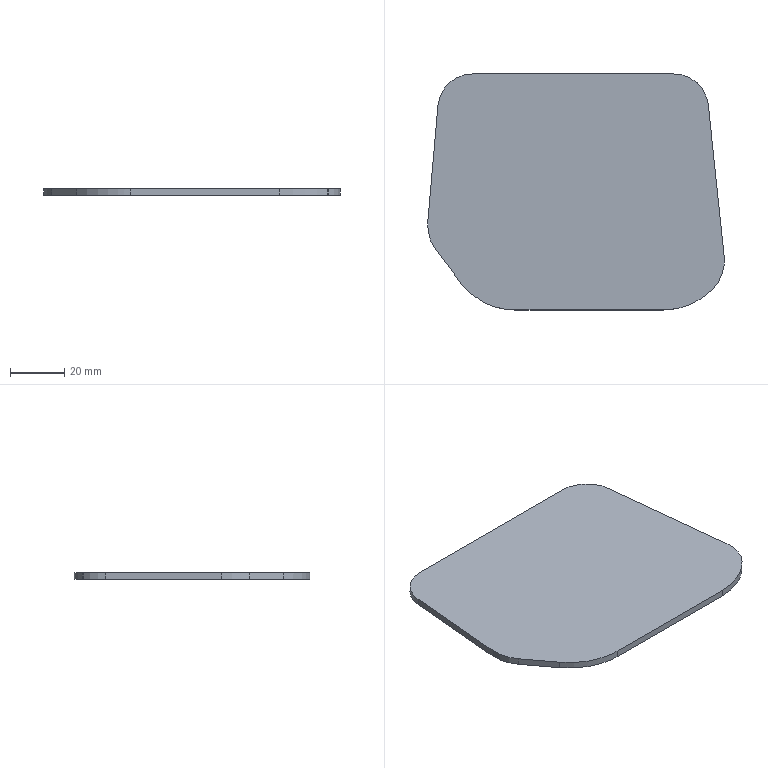Part | STEP file | lll_id402_x_t | 1 solid | 18 faces | box 109.864 x 87.36 x 2.5 mm | volume 21961 mm3 | plane 8 | cylinder 8 | other 2 | commonest cylinder face diameters 25.6 x4 30 x2 50 x2
STEP:
#1=CARTESIAN_POINT('',(3541.13,-66.264,0.00001757));
#2=VERTEX_POINT('',#1);
#3=CARTESIAN_POINT('',(3541.13,-66.264,-2.5));
#4=VERTEX_POINT('',#3);
#5=CARTESIAN_POINT('',(3541.13,-66.264,0.00001757));
#6=CARTESIAN_POINT('',(3541.13,-66.264,-0.8333));
#7=CARTESIAN_POINT('',(3541.13,-66.264,-1.667));
#8=CARTESIAN_POINT('',(3541.13,-66.264,-2.5));
#9=B_SPLINE_CURVE_WITH_KNOTS('',3,(#5,#6,#7,#8),.UNSPECIFIED.,.F.,.F.,(4,4),(0.,1.),.UNSPECIFIED.);
#10=EDGE_CURVE('',#2,#4,#9,.T.);
#11=ORIENTED_EDGE('',*,*,#10,.F.);
#12=CARTESIAN_POINT('',(3541.656,-65.782,0.00001757));
#13=VERTEX_POINT('',#12);
#14=CARTESIAN_POINT('',(3537.286,-74.341,0.00001754));
#15=CARTESIAN_POINT('',(3537.32,-73.947,0.00001754));
#16=CARTESIAN_POINT('',(3537.425,-73.162,0.00001754));
#17=CARTESIAN_POINT('',(3537.778,-71.617,0.00001754));
#18=CARTESIAN_POINT('',(3538.492,-69.763,0.00001755));
#19=CARTESIAN_POINT('',(3539.736,-67.729,0.00001755));
#20=CARTESIAN_POINT('',(3541.341,-65.967,0.00001757));
#21=CARTESIAN_POINT('',(3543.237,-64.521,0.00001758));
#22=CARTESIAN_POINT('',(3545.372,-63.46,0.0000176));
#23=CARTESIAN_POINT('',(3547.281,-62.91,0.00001761));
#24=CARTESIAN_POINT('',(3548.85,-62.692,0.00001762));
#25=CARTESIAN_POINT('',(3549.641,-62.657,0.00001763));
#26=CARTESIAN_POINT('',(3550.037,-62.657,0.00001763));
#27=B_SPLINE_CURVE_WITH_KNOTS('',3,(#14,#15,#16,#17,#18,#19,#20,#21,#22,#23,#24,#25,#26),.UNSPECIFIED.,.F.,.F.,(4,1,1,1,1,1,1,1,1,1,4),(0.,0.0625,0.125,0.25,0.375,0.5,0.625,0.75,0.875,0.9375,1.),.UNSPECIFIED.);
#28=EDGE_CURVE('',#2,#13,#27,.T.);
#29=ORIENTED_EDGE('',*,*,#28,.T.);
#30=CARTESIAN_POINT('',(3541.656,-65.782,-2.5));
#31=VERTEX_POINT('',#30);
#32=CARTESIAN_POINT('',(3541.656,-65.782,-2.5));
#33=CARTESIAN_POINT('',(3541.656,-65.782,-1.667));
#34=CARTESIAN_POINT('',(3541.656,-65.782,-0.8333));
#35=CARTESIAN_POINT('',(3541.656,-65.782,0.00001757));
#36=B_SPLINE_CURVE_WITH_KNOTS('',3,(#32,#33,#34,#35),.UNSPECIFIED.,.F.,.F.,(4,4),(0.,1.),.UNSPECIFIED.);
#37=EDGE_CURVE('',#31,#13,#36,.T.);
#38=ORIENTED_EDGE('',*,*,#37,.F.);
#39=CARTESIAN_POINT('',(3537.286,-74.341,-2.5));
#40=CARTESIAN_POINT('',(3537.32,-73.947,-2.5));
#41=CARTESIAN_POINT('',(3537.425,-73.162,-2.5));
#42=CARTESIAN_POINT('',(3537.778,-71.617,-2.5));
#43=CARTESIAN_POINT('',(3538.492,-69.763,-2.5));
#44=CARTESIAN_POINT('',(3539.736,-67.729,-2.5));
#45=CARTESIAN_POINT('',(3541.341,-65.967,-2.5));
#46=CARTESIAN_POINT('',(3543.237,-64.521,-2.5));
#47=CARTESIAN_POINT('',(3545.372,-63.46,-2.5));
#48=CARTESIAN_POINT('',(3547.281,-62.91,-2.5));
#49=CARTESIAN_POINT('',(3548.85,-62.692,-2.5));
#50=CARTESIAN_POINT('',(3549.641,-62.657,-2.5));
#51=CARTESIAN_POINT('',(3550.037,-62.657,-2.5));
#52=B_SPLINE_CURVE_WITH_KNOTS('',3,(#39,#40,#41,#42,#43,#44,#45,#46,#47,#48,#49,#50,#51),.UNSPECIFIED.,.F.,.F.,(4,1,1,1,1,1,1,1,1,1,4),(0.,0.0625,0.125,0.25,0.375,0.5,0.625,0.75,0.875,0.9375,1.),.UNSPECIFIED.);
#53=EDGE_CURVE('',#4,#31,#52,.T.);
#54=ORIENTED_EDGE('',*,*,#53,.F.);
#55=EDGE_LOOP('',(#11,#29,#38,#54));
#56=FACE_OUTER_BOUND('',#55,.T.);
#57=CARTESIAN_POINT('',(3537.286,-74.341,-2.5));
#58=CARTESIAN_POINT('',(3537.32,-73.947,-2.5));
#59=CARTESIAN_POINT('',(3537.425,-73.162,-2.5));
#60=CARTESIAN_POINT('',(3537.778,-71.617,-2.5));
#61=CARTESIAN_POINT('',(3538.492,-69.763,-2.5));
#62=CARTESIAN_POINT('',(3539.736,-67.729,-2.5));
#63=CARTESIAN_POINT('',(3541.341,-65.967,-2.5));
#64=CARTESIAN_POINT('',(3543.237,-64.521,-2.5));
#65=CARTESIAN_POINT('',(3545.372,-63.46,-2.5));
#66=CARTESIAN_POINT('',(3547.281,-62.91,-2.5));
#67=CARTESIAN_POINT('',(3548.85,-62.692,-2.5));
#68=CARTESIAN_POINT('',(3549.641,-62.657,-2.5));
#69=CARTESIAN_POINT('',(3550.037,-62.657,-2.5));
#70=B_SPLINE_CURVE_WITH_KNOTS('',3,(#57,#58,#59,#60,#61,#62,#63,#64,#65,#66,#67,#68,#69),.UNSPECIFIED.,.F.,.F.,(4,1,1,1,1,1,1,1,1,1,4),(0.,0.0625,0.125,0.25,0.375,0.5,0.625,0.75,0.875,0.9375,1.),.UNSPECIFIED.);
#71=DIRECTION('',(0.,0.000000006,1.));
#72=VECTOR('',#71,1.);
#73=SURFACE_OF_LINEAR_EXTRUSION('',#70,#72);
#74=ADVANCED_FACE('',(#56),#73,.F.);
#75=CARTESIAN_POINT('',(3632.944,-65.718,0.00001826));
#76=VERTEX_POINT('',#75);
#77=CARTESIAN_POINT('',(3632.944,-65.718,-2.5));
#78=VERTEX_POINT('',#77);
#79=CARTESIAN_POINT('',(3632.944,-65.718,0.00001826));
#80=CARTESIAN_POINT('',(3632.944,-65.718,-0.8333));
#81=CARTESIAN_POINT('',(3632.944,-65.718,-1.667));
#82=CARTESIAN_POINT('',(3632.944,-65.718,-2.5));
#83=B_SPLINE_CURVE_WITH_KNOTS('',3,(#79,#80,#81,#82),.UNSPECIFIED.,.F.,.F.,(4,4),(0.,1.),.UNSPECIFIED.);
#84=EDGE_CURVE('',#76,#78,#83,.T.);
#85=ORIENTED_EDGE('',*,*,#84,.F.);
#86=CARTESIAN_POINT('',(3633.454,-66.177,0.00001826));
#87=VERTEX_POINT('',#86);
#88=CARTESIAN_POINT('',(3624.637,-62.657,0.0000182));
#89=CARTESIAN_POINT('',(3625.028,-62.657,0.0000182));
#90=CARTESIAN_POINT('',(3625.81,-62.691,0.00001821));
#91=CARTESIAN_POINT('',(3627.361,-62.904,0.00001822));
#92=CARTESIAN_POINT('',(3629.249,-63.441,0.00001823));
#93=CARTESIAN_POINT('',(3631.364,-64.478,0.00001825));
#94=CARTESIAN_POINT('',(3633.249,-65.892,0.00001826));
#95=CARTESIAN_POINT('',(3634.852,-67.618,0.00001828));
#96=CARTESIAN_POINT('',(3636.105,-69.613,0.00001828));
#97=CARTESIAN_POINT('',(3636.836,-71.435,0.00001829));
#98=CARTESIAN_POINT('',(3637.21,-72.956,0.00001829));
#99=CARTESIAN_POINT('',(3637.326,-73.73,0.00001829));
#100=CARTESIAN_POINT('',(3637.367,-74.119,0.00001829));
#101=B_SPLINE_CURVE_WITH_KNOTS('',3,(#88,#89,#90,#91,#92,#93,#94,#95,#96,#97,#98,#99,#100),.UNSPECIFIED.,.F.,.F.,(4,1,1,1,1,1,1,1,1,1,4),(0.,0.0625,0.125,0.25,0.375,0.5,0.625,0.75,0.875,0.9375,1.),.UNSPECIFIED.);
#102=EDGE_CURVE('',#76,#87,#101,.T.);
#103=ORIENTED_EDGE('',*,*,#102,.T.);
#104=CARTESIAN_POINT('',(3633.454,-66.177,-2.5));
#105=VERTEX_POINT('',#104);
#106=CARTESIAN_POINT('',(3633.454,-66.177,-2.5));
#107=CARTESIAN_POINT('',(3633.454,-66.177,-1.667));
#108=CARTESIAN_POINT('',(3633.454,-66.177,-0.8333));
#109=CARTESIAN_POINT('',(3633.454,-66.177,0.00001826));
#110=B_SPLINE_CURVE_WITH_KNOTS('',3,(#106,#107,#108,#109),.UNSPECIFIED.,.F.,.F.,(4,4),(0.,1.),.UNSPECIFIED.);
#111=EDGE_CURVE('',#105,#87,#110,.T.);
#112=ORIENTED_EDGE('',*,*,#111,.F.);
#113=CARTESIAN_POINT('',(3624.637,-62.657,-2.5));
#114=CARTESIAN_POINT('',(3625.028,-62.657,-2.5));
#115=CARTESIAN_POINT('',(3625.81,-62.691,-2.5));
#116=CARTESIAN_POINT('',(3627.361,-62.904,-2.5));
#117=CARTESIAN_POINT('',(3629.249,-63.441,-2.5));
#118=CARTESIAN_POINT('',(3631.364,-64.478,-2.5));
#119=CARTESIAN_POINT('',(3633.249,-65.892,-2.5));
#120=CARTESIAN_POINT('',(3634.852,-67.618,-2.5));
#121=CARTESIAN_POINT('',(3636.105,-69.613,-2.5));
#122=CARTESIAN_POINT('',(3636.836,-71.435,-2.5));
#123=CARTESIAN_POINT('',(3637.21,-72.956,-2.5));
#124=CARTESIAN_POINT('',(3637.326,-73.73,-2.5));
#125=CARTESIAN_POINT('',(3637.367,-74.119,-2.5));
#126=B_SPLINE_CURVE_WITH_KNOTS('',3,(#113,#114,#115,#116,#117,#118,#119,#120,#121,#122,#123,#124,#125),.UNSPECIFIED.,.F.,.F.,(4,1,1,1,1,1,1,1,1,1,4),(0.,0.0625,0.125,0.25,0.375,0.5,0.625,0.75,0.875,0.9375,1.),.UNSPECIFIED.);
#127=EDGE_CURVE('',#78,#105,#126,.T.);
#128=ORIENTED_EDGE('',*,*,#127,.F.);
#129=EDGE_LOOP('',(#85,#103,#112,#128));
#130=FACE_OUTER_BOUND('',#129,.T.);
#131=CARTESIAN_POINT('',(3624.637,-62.657,-2.5));
#132=CARTESIAN_POINT('',(3625.028,-62.657,-2.5));
#133=CARTESIAN_POINT('',(3625.81,-62.691,-2.5));
#134=CARTESIAN_POINT('',(3627.361,-62.904,-2.5));
#135=CARTESIAN_POINT('',(3629.249,-63.441,-2.5));
#136=CARTESIAN_POINT('',(3631.364,-64.478,-2.5));
#137=CARTESIAN_POINT('',(3633.249,-65.892,-2.5));
#138=CARTESIAN_POINT('',(3634.852,-67.618,-2.5));
#139=CARTESIAN_POINT('',(3636.105,-69.613,-2.5));
#140=CARTESIAN_POINT('',(3636.836,-71.435,-2.5));
#141=CARTESIAN_POINT('',(3637.21,-72.956,-2.5));
#142=CARTESIAN_POINT('',(3637.326,-73.73,-2.5));
#143=CARTESIAN_POINT('',(3637.367,-74.119,-2.5));
#144=B_SPLINE_CURVE_WITH_KNOTS('',3,(#131,#132,#133,#134,#135,#136,#137,#138,#139,#140,#141,#142,#143),.UNSPECIFIED.,.F.,.F.,(4,1,1,1,1,1,1,1,1,1,4),(0.,0.0625,0.125,0.25,0.375,0.5,0.625,0.75,0.875,0.9375,1.),.UNSPECIFIED.);
#145=DIRECTION('',(0.,0.000000006,1.));
#146=VECTOR('',#145,1.);
#147=SURFACE_OF_LINEAR_EXTRUSION('',#144,#146);
#148=ADVANCED_FACE('',(#130),#147,.F.);
#149=CARTESIAN_POINT('',(3643.25,-130.089,-2.5));
#150=VERTEX_POINT('',#149);
#151=CARTESIAN_POINT('',(3643.25,-130.089,0.00001832));
#152=VERTEX_POINT('',#151);
#153=CARTESIAN_POINT('',(3643.25,-130.089,-7.5));
#154=DIRECTION('',(0.000000001,0.000000001,1.));
#155=VECTOR('',#154,1.);
#156=LINE('',#153,#155);
#157=EDGE_CURVE('',#150,#152,#156,.T.);
#158=ORIENTED_EDGE('',*,*,#157,.F.);
#159=CARTESIAN_POINT('',(3637.367,-74.119,-2.5));
#160=VERTEX_POINT('',#159);
#161=CARTESIAN_POINT('',(3639.152,-91.104,-2.5));
#162=DIRECTION('',(0.1045,-0.9945,0.000000001));
#163=VECTOR('',#162,1.);
#164=LINE('',#161,#163);
#165=EDGE_CURVE('',#160,#150,#164,.T.);
#166=ORIENTED_EDGE('',*,*,#165,.F.);
#167=CARTESIAN_POINT('',(3637.367,-74.119,0.0000182));
#168=VERTEX_POINT('',#167);
#169=CARTESIAN_POINT('',(3637.367,-74.119,-2.5));
#170=DIRECTION('',(0.,0.000000006,1.));
#171=VECTOR('',#170,1.);
#172=LINE('',#169,#171);
#173=EDGE_CURVE('',#160,#168,#172,.T.);
#174=ORIENTED_EDGE('',*,*,#173,.T.);
#175=CARTESIAN_POINT('',(3639.152,-91.104,0.00001831));
#176=DIRECTION('',(0.1045,-0.9945,0.000000001));
#177=VECTOR('',#176,1.);
#178=LINE('',#175,#177);
#179=EDGE_CURVE('',#168,#152,#178,.T.);
#180=ORIENTED_EDGE('',*,*,#179,.T.);
#181=EDGE_LOOP('',(#158,#166,#174,#180));
#182=FACE_OUTER_BOUND('',#181,.T.);
#183=CARTESIAN_POINT('',(3637.367,-74.119,-2.5));
#184=DIRECTION('',(-0.9945,-0.1045,0.000000001));
#185=DIRECTION('',(0.1045,-0.9945,0.));
#186=AXIS2_PLACEMENT_3D('',#183,#184,#185);
#187=PLANE('',#186);
#188=ADVANCED_FACE('',(#182),#187,.F.);
#189=CARTESIAN_POINT('',(3637.367,-74.119,-2.5));
#190=CARTESIAN_POINT('',(3637.052,-71.122,-2.5));
#191=CARTESIAN_POINT('',(3635.638,-68.253,-2.5));
#192=CARTESIAN_POINT('',(3633.454,-66.177,-2.5));
#193=B_SPLINE_CURVE_WITH_KNOTS('',3,(#189,#190,#191,#192),.UNSPECIFIED.,.F.,.F.,(4,4),(0.,1.),.UNSPECIFIED.);
#194=EDGE_CURVE('',#160,#105,#193,.T.);
#195=ORIENTED_EDGE('',*,*,#194,.F.);
#196=ORIENTED_EDGE('',*,*,#165,.T.);
#197=CARTESIAN_POINT('',(3638.938,-142.263,-2.5));
#198=VERTEX_POINT('',#197);
#199=CARTESIAN_POINT('',(3628.332,-131.657,-2.5));
#200=DIRECTION('',(-0.000000008,0.,1.));
#201=DIRECTION('',(1.,0.,0.000000008));
#202=AXIS2_PLACEMENT_3D('',#199,#200,#201);
#203=CIRCLE('',#202,15.);
#204=EDGE_CURVE('',#198,#150,#203,.T.);
#205=ORIENTED_EDGE('',*,*,#204,.F.);
#206=CARTESIAN_POINT('',(3638.507,-142.694,-2.5));
#207=VERTEX_POINT('',#206);
#208=CARTESIAN_POINT('',(3596.229,-184.973,-2.5));
#209=DIRECTION('',(0.7071,0.7071,0.000000005));
#210=VECTOR('',#209,1.);
#211=LINE('',#208,#210);
#212=EDGE_CURVE('',#207,#198,#211,.T.);
#213=ORIENTED_EDGE('',*,*,#212,.F.);
#214=CARTESIAN_POINT('',(3620.83,-150.017,-2.5));
#215=VERTEX_POINT('',#214);
#216=CARTESIAN_POINT('',(3620.83,-125.017,-2.5));
#217=DIRECTION('',(-0.000000008,0.,1.));
#218=DIRECTION('',(1.,0.,0.000000008));
#219=AXIS2_PLACEMENT_3D('',#216,#217,#218);
#220=CIRCLE('',#219,25.);
#221=EDGE_CURVE('',#215,#207,#220,.T.);
#222=ORIENTED_EDGE('',*,*,#221,.F.);
#223=CARTESIAN_POINT('',(3565.78,-150.017,-2.5));
#224=VERTEX_POINT('',#223);
#225=CARTESIAN_POINT('',(3581.149,-150.017,-2.5));
#226=DIRECTION('',(-1.,0.,-0.000000008));
#227=VECTOR('',#226,1.);
#228=LINE('',#225,#227);
#229=EDGE_CURVE('',#215,#224,#228,.T.);
#230=ORIENTED_EDGE('',*,*,#229,.T.);
#231=CARTESIAN_POINT('',(3545.814,-140.062,-2.5));
#232=VERTEX_POINT('',#231);
#233=CARTESIAN_POINT('',(3545.814,-140.062,-2.5));
#234=CARTESIAN_POINT('',(3548.134,-143.14,-2.5));
#235=CARTESIAN_POINT('',(3551.176,-145.67,-2.5));
#236=CARTESIAN_POINT('',(3558.074,-149.11,-2.5));
#237=CARTESIAN_POINT('',(3561.926,-150.017,-2.5));
#238=CARTESIAN_POINT('',(3565.78,-150.017,-2.5));
#239=B_SPLINE_CURVE_WITH_KNOTS('',3,(#233,#234,#235,#236,#237,#238),.UNSPECIFIED.,.F.,.F.,(4,2,4),(0.,0.5,1.),.UNSPECIFIED.);
#240=EDGE_CURVE('',#232,#224,#239,.T.);
#241=ORIENTED_EDGE('',*,*,#240,.F.);
#242=CARTESIAN_POINT('',(3536.486,-127.684,-2.5));
#243=VERTEX_POINT('',#242);
#244=CARTESIAN_POINT('',(3541.15,-133.873,-2.5));
#245=DIRECTION('',(-0.6018,0.7986,-0.000000005));
#246=VECTOR('',#245,1.);
#247=LINE('',#244,#246);
#248=EDGE_CURVE('',#232,#243,#247,.T.);
#249=ORIENTED_EDGE('',*,*,#248,.T.);
#250=CARTESIAN_POINT('',(3533.523,-117.349,-2.5));
#251=VERTEX_POINT('',#250);
#252=CARTESIAN_POINT('',(3533.523,-117.349,-2.5));
#253=CARTESIAN_POINT('',(3533.204,-121.,-2.5));
#254=CARTESIAN_POINT('',(3534.281,-124.757,-2.5));
#255=CARTESIAN_POINT('',(3536.486,-127.684,-2.5));
#256=B_SPLINE_CURVE_WITH_KNOTS('',3,(#252,#253,#254,#255),.UNSPECIFIED.,.F.,.F.,(4,4),(0.,1.),.UNSPECIFIED.);
#257=EDGE_CURVE('',#251,#243,#256,.T.);
#258=ORIENTED_EDGE('',*,*,#257,.F.);
#259=CARTESIAN_POINT('',(3537.286,-74.341,-2.5));
#260=VERTEX_POINT('',#259);
#261=CARTESIAN_POINT('',(3535.404,-95.845,-2.5));
#262=DIRECTION('',(0.08716,0.9962,0.000000001));
#263=VECTOR('',#262,1.);
#264=LINE('',#261,#263);
#265=EDGE_CURVE('',#251,#260,#264,.T.);
#266=ORIENTED_EDGE('',*,*,#265,.T.);
#267=CARTESIAN_POINT('',(3541.13,-66.264,-2.5));
#268=CARTESIAN_POINT('',(3538.942,-68.384,-2.5));
#269=CARTESIAN_POINT('',(3537.551,-71.307,-2.5));
#270=CARTESIAN_POINT('',(3537.286,-74.341,-2.5));
#271=B_SPLINE_CURVE_WITH_KNOTS('',3,(#267,#268,#269,#270),.UNSPECIFIED.,.F.,.F.,(4,4),(0.,1.),.UNSPECIFIED.);
#272=EDGE_CURVE('',#4,#260,#271,.T.);
#273=ORIENTED_EDGE('',*,*,#272,.F.);
#274=ORIENTED_EDGE('',*,*,#53,.T.);
#275=CARTESIAN_POINT('',(3550.037,-62.657,-2.5));
#276=VERTEX_POINT('',#275);
#277=CARTESIAN_POINT('',(3550.037,-62.657,-2.5));
#278=CARTESIAN_POINT('',(3546.991,-62.657,-2.5));
#279=CARTESIAN_POINT('',(3543.958,-63.788,-2.5));
#280=CARTESIAN_POINT('',(3541.656,-65.782,-2.5));
#281=B_SPLINE_CURVE_WITH_KNOTS('',3,(#277,#278,#279,#280),.UNSPECIFIED.,.F.,.F.,(4,4),(0.,1.),.UNSPECIFIED.);
#282=EDGE_CURVE('',#276,#31,#281,.T.);
#283=ORIENTED_EDGE('',*,*,#282,.F.);
#284=CARTESIAN_POINT('',(3624.637,-62.657,-2.5));
#285=VERTEX_POINT('',#284);
#286=CARTESIAN_POINT('',(3587.337,-62.657,-2.5));
#287=DIRECTION('',(1.,0.,0.000000008));
#288=VECTOR('',#287,1.);
#289=LINE('',#286,#288);
#290=EDGE_CURVE('',#276,#285,#289,.T.);
#291=ORIENTED_EDGE('',*,*,#290,.T.);
#292=CARTESIAN_POINT('',(3632.944,-65.718,-2.5));
#293=CARTESIAN_POINT('',(3630.651,-63.763,-2.5));
#294=CARTESIAN_POINT('',(3627.65,-62.657,-2.5));
#295=CARTESIAN_POINT('',(3624.637,-62.657,-2.5));
#296=B_SPLINE_CURVE_WITH_KNOTS('',3,(#292,#293,#294,#295),.UNSPECIFIED.,.F.,.F.,(4,4),(0.,1.),.UNSPECIFIED.);
#297=EDGE_CURVE('',#78,#285,#296,.T.);
#298=ORIENTED_EDGE('',*,*,#297,.F.);
#299=ORIENTED_EDGE('',*,*,#127,.T.);
#300=EDGE_LOOP('',(#195,#196,#205,#213,#222,#230,#241,#249,#258,#266,#273,#274,#283,#291,#298,#299));
#301=FACE_OUTER_BOUND('',#300,.T.);
#302=CARTESIAN_POINT('',(3534.047,-122.791,-2.5));
#303=DIRECTION('',(-0.000000008,0.,1.));
#304=DIRECTION('',(-1.,0.,-0.000000008));
#305=AXIS2_PLACEMENT_3D('',#302,#303,#304);
#306=PLANE('',#305);
#307=ADVANCED_FACE('',(#301),#306,.F.);
#308=ORIENTED_EDGE('',*,*,#179,.F.);
#309=CARTESIAN_POINT('',(3637.367,-74.119,0.0000183));
#310=CARTESIAN_POINT('',(3637.051,-71.113,0.00001829));
#311=CARTESIAN_POINT('',(3635.645,-68.26,0.00001828));
#312=CARTESIAN_POINT('',(3633.454,-66.177,0.00001827));
#313=B_SPLINE_CURVE_WITH_KNOTS('',3,(#309,#310,#311,#312),.UNSPECIFIED.,.F.,.F.,(4,4),(0.,1.),.UNSPECIFIED.);
#314=EDGE_CURVE('',#168,#87,#313,.T.);
#315=ORIENTED_EDGE('',*,*,#314,.T.);
#316=ORIENTED_EDGE('',*,*,#102,.F.);
#317=CARTESIAN_POINT('',(3624.637,-62.657,0.0000182));
#318=VERTEX_POINT('',#317);
#319=CARTESIAN_POINT('',(3632.944,-65.718,0.00001826));
#320=CARTESIAN_POINT('',(3630.645,-63.757,0.00001824));
#321=CARTESIAN_POINT('',(3627.66,-62.657,0.00001822));
#322=CARTESIAN_POINT('',(3624.637,-62.657,0.0000182));
#323=B_SPLINE_CURVE_WITH_KNOTS('',3,(#319,#320,#321,#322),.UNSPECIFIED.,.F.,.F.,(4,4),(0.,1.),.UNSPECIFIED.);
#324=EDGE_CURVE('',#76,#318,#323,.T.);
#325=ORIENTED_EDGE('',*,*,#324,.T.);
#326=CARTESIAN_POINT('',(3550.037,-62.657,0.00001763));
#327=VERTEX_POINT('',#326);
#328=CARTESIAN_POINT('',(3587.337,-62.657,0.00001792));
#329=DIRECTION('',(1.,0.,0.000000008));
#330=VECTOR('',#329,1.);
#331=LINE('',#328,#330);
#332=EDGE_CURVE('',#327,#318,#331,.T.);
#333=ORIENTED_EDGE('',*,*,#332,.F.);
#334=CARTESIAN_POINT('',(3550.037,-62.657,0.00001763));
#335=CARTESIAN_POINT('',(3546.982,-62.657,0.00001761));
#336=CARTESIAN_POINT('',(3543.966,-63.781,0.00001759));
#337=CARTESIAN_POINT('',(3541.656,-65.782,0.00001757));
#338=B_SPLINE_CURVE_WITH_KNOTS('',3,(#334,#335,#336,#337),.UNSPECIFIED.,.F.,.F.,(4,4),(0.,1.),.UNSPECIFIED.);
#339=EDGE_CURVE('',#327,#13,#338,.T.);
#340=ORIENTED_EDGE('',*,*,#339,.T.);
#341=ORIENTED_EDGE('',*,*,#28,.F.);
#342=CARTESIAN_POINT('',(3537.286,-74.341,0.00001754));
#343=VERTEX_POINT('',#342);
#344=CARTESIAN_POINT('',(3541.13,-66.264,0.00001757));
#345=CARTESIAN_POINT('',(3538.936,-68.39,0.00001755));
#346=CARTESIAN_POINT('',(3537.552,-71.296,0.00001754));
#347=CARTESIAN_POINT('',(3537.286,-74.341,0.00001754));
#348=B_SPLINE_CURVE_WITH_KNOTS('',3,(#344,#345,#346,#347),.UNSPECIFIED.,.F.,.F.,(4,4),(0.,1.),.UNSPECIFIED.);
#349=EDGE_CURVE('',#2,#343,#348,.T.);
#350=ORIENTED_EDGE('',*,*,#349,.T.);
#351=CARTESIAN_POINT('',(3533.523,-117.349,0.00001762));
#352=VERTEX_POINT('',#351);
#353=CARTESIAN_POINT('',(3535.404,-95.845,0.00001752));
#354=DIRECTION('',(0.08716,0.9962,0.000000001));
#355=VECTOR('',#354,1.);
#356=LINE('',#353,#355);
#357=EDGE_CURVE('',#352,#343,#356,.T.);
#358=ORIENTED_EDGE('',*,*,#357,.F.);
#359=CARTESIAN_POINT('',(3536.486,-127.684,0.00001753));
#360=VERTEX_POINT('',#359);
#361=CARTESIAN_POINT('',(3533.523,-117.349,0.00001751));
#362=CARTESIAN_POINT('',(3533.203,-121.011,0.0000175));
#363=CARTESIAN_POINT('',(3534.273,-124.746,0.00001751));
#364=CARTESIAN_POINT('',(3536.486,-127.684,0.00001753));
#365=B_SPLINE_CURVE_WITH_KNOTS('',3,(#361,#362,#363,#364),.UNSPECIFIED.,.F.,.F.,(4,4),(0.,1.),.UNSPECIFIED.);
#366=EDGE_CURVE('',#352,#360,#365,.T.);
#367=ORIENTED_EDGE('',*,*,#366,.T.);
#368=CARTESIAN_POINT('',(3545.814,-140.062,0.00001775));
#369=VERTEX_POINT('',#368);
#370=CARTESIAN_POINT('',(3541.15,-133.873,0.00001757));
#371=DIRECTION('',(-0.6018,0.7986,-0.000000005));
#372=VECTOR('',#371,1.);
#373=LINE('',#370,#372);
#374=EDGE_CURVE('',#369,#360,#373,.T.);
#375=ORIENTED_EDGE('',*,*,#374,.F.);
#376=CARTESIAN_POINT('',(3565.78,-150.017,0.00001775));
#377=VERTEX_POINT('',#376);
#378=CARTESIAN_POINT('',(3545.814,-140.062,0.0000176));
#379=CARTESIAN_POINT('',(3548.144,-143.154,0.00001762));
#380=CARTESIAN_POINT('',(3551.161,-145.663,0.00001764));
#381=CARTESIAN_POINT('',(3558.089,-149.117,0.00001769));
#382=CARTESIAN_POINT('',(3561.907,-150.016,0.00001772));
#383=CARTESIAN_POINT('',(3565.78,-150.017,0.00001775));
#384=B_SPLINE_CURVE_WITH_KNOTS('',3,(#378,#379,#380,#381,#382,#383),.UNSPECIFIED.,.F.,.F.,(4,2,4),(0.,0.5,1.),.UNSPECIFIED.);
#385=EDGE_CURVE('',#369,#377,#384,.T.);
#386=ORIENTED_EDGE('',*,*,#385,.T.);
#387=CARTESIAN_POINT('',(3620.83,-150.017,0.00001817));
#388=VERTEX_POINT('',#387);
#389=CARTESIAN_POINT('',(3581.149,-150.017,0.00001787));
#390=DIRECTION('',(-1.,0.,-0.000000008));
#391=VECTOR('',#390,1.);
#392=LINE('',#389,#391);
#393=EDGE_CURVE('',#388,#377,#392,.T.);
#394=ORIENTED_EDGE('',*,*,#393,.F.);
#395=CARTESIAN_POINT('',(3638.507,-142.694,0.00001831));
#396=VERTEX_POINT('',#395);
#397=CARTESIAN_POINT('',(3620.83,-125.017,0.00001817));
#398=DIRECTION('',(0.000000008,0.,-1.));
#399=DIRECTION('',(1.,0.,0.000000008));
#400=AXIS2_PLACEMENT_3D('',#397,#398,#399);
#401=CIRCLE('',#400,25.);
#402=EDGE_CURVE('',#396,#388,#401,.T.);
#403=ORIENTED_EDGE('',*,*,#402,.F.);
#404=CARTESIAN_POINT('',(3638.938,-142.263,0.00001831));
#405=VERTEX_POINT('',#404);
#406=CARTESIAN_POINT('',(3596.229,-184.973,0.00001798));
#407=DIRECTION('',(0.7071,0.7071,0.000000005));
#408=VECTOR('',#407,1.);
#409=LINE('',#406,#408);
#410=EDGE_CURVE('',#396,#405,#409,.T.);
#411=ORIENTED_EDGE('',*,*,#410,.T.);
#412=CARTESIAN_POINT('',(3628.332,-131.657,0.00001823));
#413=DIRECTION('',(-0.000000008,0.,1.));
#414=DIRECTION('',(1.,0.,0.000000008));
#415=AXIS2_PLACEMENT_3D('',#412,#413,#414);
#416=CIRCLE('',#415,15.);
#417=EDGE_CURVE('',#405,#152,#416,.T.);
#418=ORIENTED_EDGE('',*,*,#417,.T.);
#419=EDGE_LOOP('',(#308,#315,#316,#325,#333,#340,#341,#350,#358,#367,#375,#386,#394,#403,#411,#418));
#420=FACE_OUTER_BOUND('',#419,.T.);
#421=CARTESIAN_POINT('',(3534.047,-122.791,0.00001751));
#422=DIRECTION('',(-0.000000008,0.,1.));
#423=DIRECTION('',(-1.,0.,-0.000000008));
#424=AXIS2_PLACEMENT_3D('',#421,#422,#423);
#425=PLANE('',#424);
#426=ADVANCED_FACE('',(#420),#425,.T.);
#427=ORIENTED_EDGE('',*,*,#374,.T.);
#428=CARTESIAN_POINT('',(3536.486,-127.684,-2.5));
#429=DIRECTION('',(0.,0.000000006,1.));
#430=VECTOR('',#429,1.);
#431=LINE('',#428,#430);
#432=EDGE_CURVE('',#243,#360,#431,.T.);
#433=ORIENTED_EDGE('',*,*,#432,.F.);
#434=ORIENTED_EDGE('',*,*,#248,.F.);
#435=CARTESIAN_POINT('',(3545.814,-140.062,-2.5));
#436=DIRECTION('',(0.,0.000000006,1.));
#437=VECTOR('',#436,1.);
#438=LINE('',#435,#437);
#439=EDGE_CURVE('',#232,#369,#438,.T.);
#440=ORIENTED_EDGE('',*,*,#439,.T.);
#441=EDGE_LOOP('',(#427,#433,#434,#440));
#442=FACE_OUTER_BOUND('',#441,.T.);
#443=CARTESIAN_POINT('',(3545.814,-140.062,-2.5));
#444=DIRECTION('',(0.7986,0.6018,-0.000000003));
#445=DIRECTION('',(-0.6018,0.7986,0.));
#446=AXIS2_PLACEMENT_3D('',#443,#444,#445);
#447=PLANE('',#446);
#448=ADVANCED_FACE('',(#442),#447,.F.);
#449=ORIENTED_EDGE('',*,*,#357,.T.);
#450=CARTESIAN_POINT('',(3537.286,-74.341,-2.5));
#451=DIRECTION('',(0.,0.000000006,1.));
#452=VECTOR('',#451,1.);
#453=LINE('',#450,#452);
#454=EDGE_CURVE('',#260,#343,#453,.T.);
#455=ORIENTED_EDGE('',*,*,#454,.F.);
#456=ORIENTED_EDGE('',*,*,#265,.F.);
#457=CARTESIAN_POINT('',(3533.523,-117.349,-2.5));
#458=DIRECTION('',(0.,0.000000006,1.));
#459=VECTOR('',#458,1.);
#460=LINE('',#457,#459);
#461=EDGE_CURVE('',#251,#352,#460,.T.);
#462=ORIENTED_EDGE('',*,*,#461,.T.);
#463=EDGE_LOOP('',(#449,#455,#456,#462));
#464=FACE_OUTER_BOUND('',#463,.T.);
#465=CARTESIAN_POINT('',(3533.523,-117.349,-2.5));
#466=DIRECTION('',(0.9962,-0.08716,0.));
#467=DIRECTION('',(0.08716,0.9962,0.));
#468=AXIS2_PLACEMENT_3D('',#465,#466,#467);
#469=PLANE('',#468);
#470=ADVANCED_FACE('',(#464),#469,.F.);
#471=ORIENTED_EDGE('',*,*,#332,.T.);
#472=CARTESIAN_POINT('',(3624.637,-62.657,-2.5));
#473=DIRECTION('',(0.,0.000000006,1.));
#474=VECTOR('',#473,1.);
#475=LINE('',#472,#474);
#476=EDGE_CURVE('',#285,#318,#475,.T.);
#477=ORIENTED_EDGE('',*,*,#476,.F.);
#478=ORIENTED_EDGE('',*,*,#290,.F.);
#479=CARTESIAN_POINT('',(3550.037,-62.657,-2.5));
#480=DIRECTION('',(0.,0.000000006,1.));
#481=VECTOR('',#480,1.);
#482=LINE('',#479,#481);
#483=EDGE_CURVE('',#276,#327,#482,.T.);
#484=ORIENTED_EDGE('',*,*,#483,.T.);
#485=EDGE_LOOP('',(#471,#477,#478,#484));
#486=FACE_OUTER_BOUND('',#485,.T.);
#487=CARTESIAN_POINT('',(3550.037,-62.657,-2.5));
#488=DIRECTION('',(0.,-1.,0.000000006));
#489=DIRECTION('',(0.,0.000000006,1.));
#490=AXIS2_PLACEMENT_3D('',#487,#488,#489);
#491=PLANE('',#490);
#492=ADVANCED_FACE('',(#486),#491,.F.);
#493=ORIENTED_EDGE('',*,*,#229,.F.);
#494=CARTESIAN_POINT('',(3620.83,-150.017,-7.5));
#495=DIRECTION('',(-0.000000001,-0.000000001,-1.));
#496=VECTOR('',#495,1.);
#497=LINE('',#494,#496);
#498=EDGE_CURVE('',#388,#215,#497,.T.);
#499=ORIENTED_EDGE('',*,*,#498,.F.);
#500=ORIENTED_EDGE('',*,*,#393,.T.);
#501=CARTESIAN_POINT('',(3565.78,-150.017,-2.5));
#502=DIRECTION('',(0.,0.000000006,1.));
#503=VECTOR('',#502,1.);
#504=LINE('',#501,#503);
#505=EDGE_CURVE('',#224,#377,#504,.T.);
#506=ORIENTED_EDGE('',*,*,#505,.F.);
#507=EDGE_LOOP('',(#493,#499,#500,#506));
#508=FACE_OUTER_BOUND('',#507,.T.);
#509=CARTESIAN_POINT('',(3596.517,-150.017,-2.5));
#510=DIRECTION('',(0.,1.,-0.000000006));
#511=DIRECTION('',(0.,-0.000000006,-1.));
#512=AXIS2_PLACEMENT_3D('',#509,#510,#511);
#513=PLANE('',#512);
#514=ADVANCED_FACE('',(#508),#513,.F.);
#515=CARTESIAN_POINT('',(3638.507,-142.694,-7.5));
#516=DIRECTION('',(0.000000001,0.000000001,1.));
#517=VECTOR('',#516,1.);
#518=LINE('',#515,#517);
#519=EDGE_CURVE('',#207,#396,#518,.T.);
#520=ORIENTED_EDGE('',*,*,#519,.F.);
#521=ORIENTED_EDGE('',*,*,#212,.T.);
#522=CARTESIAN_POINT('',(3638.938,-142.263,-7.5));
#523=DIRECTION('',(0.000000001,0.000000001,1.));
#524=VECTOR('',#523,1.);
#525=LINE('',#522,#524);
#526=EDGE_CURVE('',#198,#405,#525,.T.);
#527=ORIENTED_EDGE('',*,*,#526,.T.);
#528=ORIENTED_EDGE('',*,*,#410,.F.);
#529=EDGE_LOOP('',(#520,#521,#527,#528));
#530=FACE_OUTER_BOUND('',#529,.T.);
#531=CARTESIAN_POINT('',(3638.507,-142.694,-7.5));
#532=DIRECTION('',(0.7071,-0.7071,0.));
#533=DIRECTION('',(0.7071,0.7071,0.));
#534=AXIS2_PLACEMENT_3D('',#531,#532,#533);
#535=PLANE('',#534);
#536=ADVANCED_FACE('',(#530),#535,.T.);
#537=ORIENTED_EDGE('',*,*,#498,.T.);
#538=ORIENTED_EDGE('',*,*,#221,.T.);
#539=ORIENTED_EDGE('',*,*,#519,.T.);
#540=ORIENTED_EDGE('',*,*,#402,.T.);
#541=EDGE_LOOP('',(#537,#538,#539,#540));
#542=FACE_OUTER_BOUND('',#541,.T.);
#543=CARTESIAN_POINT('',(3620.83,-125.017,-7.5));
#544=DIRECTION('',(0.000000001,0.000000001,1.));
#545=DIRECTION('',(1.,0.,-0.000000001));
#546=AXIS2_PLACEMENT_3D('',#543,#544,#545);
#547=CYLINDRICAL_SURFACE('',#546,25.);
#548=ADVANCED_FACE('',(#542),#547,.T.);
#549=ORIENTED_EDGE('',*,*,#526,.F.);
#550=ORIENTED_EDGE('',*,*,#204,.T.);
#551=ORIENTED_EDGE('',*,*,#157,.T.);
#552=ORIENTED_EDGE('',*,*,#417,.F.);
#553=EDGE_LOOP('',(#549,#550,#551,#552));
#554=FACE_OUTER_BOUND('',#553,.T.);
#555=CARTESIAN_POINT('',(3628.332,-131.657,-7.5));
#556=DIRECTION('',(0.000000001,0.000000001,1.));
#557=DIRECTION('',(1.,0.,-0.000000001));
#558=AXIS2_PLACEMENT_3D('',#555,#556,#557);
#559=CYLINDRICAL_SURFACE('',#558,15.);
#560=ADVANCED_FACE('',(#554),#559,.T.);
#561=ORIENTED_EDGE('',*,*,#439,.F.);
#562=ORIENTED_EDGE('',*,*,#240,.T.);
#563=ORIENTED_EDGE('',*,*,#505,.T.);
#564=ORIENTED_EDGE('',*,*,#385,.F.);
#565=EDGE_LOOP('',(#561,#562,#563,#564));
#566=FACE_OUTER_BOUND('',#565,.T.);
#567=CARTESIAN_POINT('',(3565.78,-125.017,-7.5));
#568=DIRECTION('',(0.000000001,0.000000001,1.));
#569=DIRECTION('',(1.,0.,-0.000000001));
#570=AXIS2_PLACEMENT_3D('',#567,#568,#569);
#571=CYLINDRICAL_SURFACE('',#570,25.);
#572=ADVANCED_FACE('',(#566),#571,.T.);
#573=ORIENTED_EDGE('',*,*,#461,.F.);
#574=ORIENTED_EDGE('',*,*,#257,.T.);
#575=ORIENTED_EDGE('',*,*,#432,.T.);
#576=ORIENTED_EDGE('',*,*,#366,.F.);
#577=EDGE_LOOP('',(#573,#574,#575,#576));
#578=FACE_OUTER_BOUND('',#577,.T.);
#579=CARTESIAN_POINT('',(3548.466,-118.657,-7.5));
#580=DIRECTION('',(0.000000001,0.000000001,1.));
#581=DIRECTION('',(1.,0.,-0.000000001));
#582=AXIS2_PLACEMENT_3D('',#579,#580,#581);
#583=CYLINDRICAL_SURFACE('',#582,15.);
#584=ADVANCED_FACE('',(#578),#583,.T.);
#585=ORIENTED_EDGE('',*,*,#10,.T.);
#586=ORIENTED_EDGE('',*,*,#272,.T.);
#587=ORIENTED_EDGE('',*,*,#454,.T.);
#588=ORIENTED_EDGE('',*,*,#349,.F.);
#589=EDGE_LOOP('',(#585,#586,#587,#588));
#590=FACE_OUTER_BOUND('',#589,.T.);
#591=CARTESIAN_POINT('',(3550.037,-75.457,-7.5));
#592=DIRECTION('',(0.000000001,0.000000001,1.));
#593=DIRECTION('',(1.,0.,-0.000000001));
#594=AXIS2_PLACEMENT_3D('',#591,#592,#593);
#595=CYLINDRICAL_SURFACE('',#594,12.8);
#596=ADVANCED_FACE('',(#590),#595,.T.);
#597=ORIENTED_EDGE('',*,*,#483,.F.);
#598=ORIENTED_EDGE('',*,*,#282,.T.);
#599=ORIENTED_EDGE('',*,*,#37,.T.);
#600=ORIENTED_EDGE('',*,*,#339,.F.);
#601=EDGE_LOOP('',(#597,#598,#599,#600));
#602=FACE_OUTER_BOUND('',#601,.T.);
#603=CARTESIAN_POINT('',(3550.037,-75.457,-7.5));
#604=DIRECTION('',(0.000000001,0.000000001,1.));
#605=DIRECTION('',(1.,0.,-0.000000001));
#606=AXIS2_PLACEMENT_3D('',#603,#604,#605);
#607=CYLINDRICAL_SURFACE('',#606,12.8);
#608=ADVANCED_FACE('',(#602),#607,.T.);
#609=ORIENTED_EDGE('',*,*,#84,.T.);
#610=ORIENTED_EDGE('',*,*,#297,.T.);
#611=ORIENTED_EDGE('',*,*,#476,.T.);
#612=ORIENTED_EDGE('',*,*,#324,.F.);
#613=EDGE_LOOP('',(#609,#610,#611,#612));
#614=FACE_OUTER_BOUND('',#613,.T.);
#615=CARTESIAN_POINT('',(3624.637,-75.457,-7.5));
#616=DIRECTION('',(0.000000001,0.000000001,1.));
#617=DIRECTION('',(1.,0.,-0.000000001));
#618=AXIS2_PLACEMENT_3D('',#615,#616,#617);
#619=CYLINDRICAL_SURFACE('',#618,12.8);
#620=ADVANCED_FACE('',(#614),#619,.T.);
#621=ORIENTED_EDGE('',*,*,#173,.F.);
#622=ORIENTED_EDGE('',*,*,#194,.T.);
#623=ORIENTED_EDGE('',*,*,#111,.T.);
#624=ORIENTED_EDGE('',*,*,#314,.F.);
#625=EDGE_LOOP('',(#621,#622,#623,#624));
#626=FACE_OUTER_BOUND('',#625,.T.);
#627=CARTESIAN_POINT('',(3624.637,-75.457,-7.5));
#628=DIRECTION('',(0.000000001,0.000000001,1.));
#629=DIRECTION('',(1.,0.,-0.000000001));
#630=AXIS2_PLACEMENT_3D('',#627,#628,#629);
#631=CYLINDRICAL_SURFACE('',#630,12.8);
#632=ADVANCED_FACE('',(#626),#631,.T.);
#633=CLOSED_SHELL('',(#74,#148,#188,#307,#426,#448,#470,#492,#514,#536,#548,#560,#572,#584,#596,#608,#620,#632));
#634=MANIFOLD_SOLID_BREP('',#633);
#635=(LENGTH_UNIT()NAMED_UNIT(*)SI_UNIT(.MILLI.,.METRE.));
#636=UNCERTAINTY_MEASURE_WITH_UNIT(LENGTH_MEASURE(0.0508),#635,'','');
#637=(NAMED_UNIT(*)PLANE_ANGLE_UNIT()SI_UNIT($,.RADIAN.));
#638=PLANE_ANGLE_MEASURE_WITH_UNIT(PLANE_ANGLE_MEASURE(0.01745),#637);
#639=DIMENSIONAL_EXPONENTS(0.,0.,0.,0.,0.,0.,0.);
#640=(CONVERSION_BASED_UNIT('DEGREE',#638)NAMED_UNIT(#639)PLANE_ANGLE_UNIT());
#641=(NAMED_UNIT(*)SI_UNIT($,.STERADIAN.)SOLID_ANGLE_UNIT());
#642=(GEOMETRIC_REPRESENTATION_CONTEXT(3)GLOBAL_UNCERTAINTY_ASSIGNED_CONTEXT((#636))GLOBAL_UNIT_ASSIGNED_CONTEXT((#635,#640,#641))REPRESENTATION_CONTEXT('',''));
#643=ADVANCED_BREP_SHAPE_REPRESENTATION('',(#634),#642);